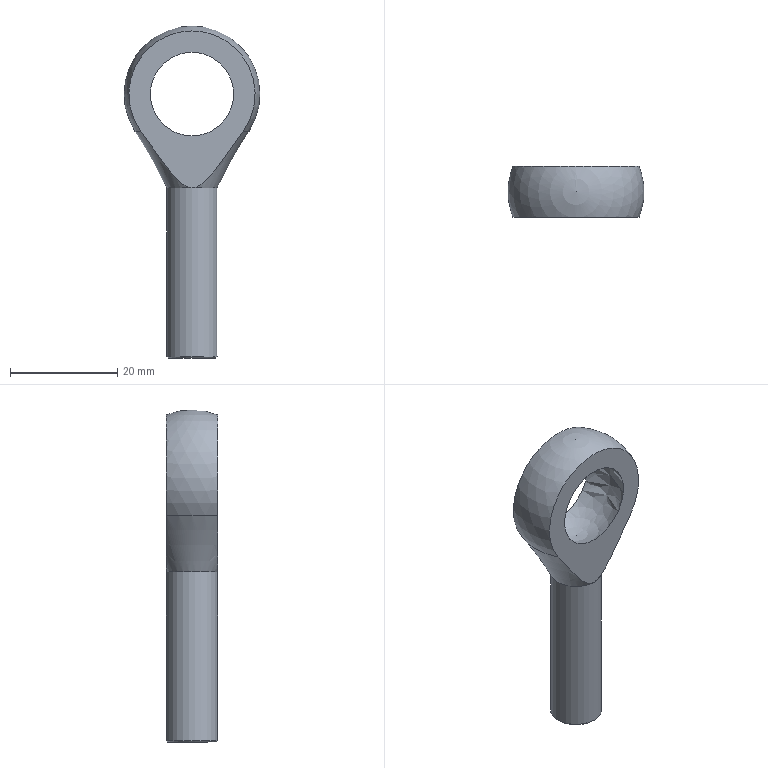Part | NX | features solid 2 | 1 solid | 9 faces | box 25.4 x 9.525 x 61.925 mm | volume 5244 mm3 | plane 3 | torus 2 | sphere 2 | cylinder 1 | cone 1 | commonest cylinder face diameters 9.525 x1
STEP:
#1=CARTESIAN_POINT('',(0.,4.763,-17.475));
#2=VERTEX_POINT('',#1);
#3=CARTESIAN_POINT('',(0.,-4.763,-17.475));
#4=VERTEX_POINT('',#3);
#5=CARTESIAN_POINT('',(0.,0.,-17.475));
#6=DIRECTION('',(0.,0.,-1.));
#7=DIRECTION('',(0.,1.,0.));
#8=AXIS2_PLACEMENT_3D('',#5,#6,#7);
#9=CIRCLE('',#8,4.763);
#10=EDGE_CURVE('',#2,#4,#9,.T.);
#11=ORIENTED_EDGE('',*,*,#10,.F.);
#12=CARTESIAN_POINT('',(9.513,4.763,-6.936));
#13=VERTEX_POINT('',#12);
#14=CARTESIAN_POINT('',(0.,4.763,-17.475));
#15=CARTESIAN_POINT('',(0.618,4.763,-17.475));
#16=CARTESIAN_POINT('',(1.763,4.763,-16.939));
#17=CARTESIAN_POINT('',(3.496,4.763,-15.237));
#18=CARTESIAN_POINT('',(5.308,4.763,-12.838));
#19=CARTESIAN_POINT('',(7.401,4.763,-9.877));
#20=CARTESIAN_POINT('',(8.802,4.763,-7.911));
#21=CARTESIAN_POINT('',(9.513,4.763,-6.936));
#22=B_SPLINE_CURVE_WITH_KNOTS('',3,(#14,#15,#16,#17,#18,#19,#20,#21),.UNSPECIFIED.,.F.,.F.,(4,1,1,1,1,4),(0.,0.001824,0.003648,0.007295,0.01094,0.01459),.UNSPECIFIED.);
#23=EDGE_CURVE('',#2,#13,#22,.T.);
#24=ORIENTED_EDGE('',*,*,#23,.T.);
#25=CARTESIAN_POINT('',(9.513,-4.763,-6.936));
#26=VERTEX_POINT('',#25);
#27=CARTESIAN_POINT('',(0.,0.,-6.936));
#28=DIRECTION('',(0.,0.,-1.));
#29=DIRECTION('',(0.,1.,0.));
#30=AXIS2_PLACEMENT_3D('',#27,#28,#29);
#31=CIRCLE('',#30,10.639);
#32=EDGE_CURVE('',#13,#26,#31,.T.);
#33=ORIENTED_EDGE('',*,*,#32,.T.);
#34=CARTESIAN_POINT('',(9.513,-4.763,-6.936));
#35=CARTESIAN_POINT('',(8.802,-4.763,-7.912));
#36=CARTESIAN_POINT('',(7.398,-4.763,-9.88));
#37=CARTESIAN_POINT('',(5.313,-4.763,-12.837));
#38=CARTESIAN_POINT('',(3.47,-4.763,-15.258));
#39=CARTESIAN_POINT('',(1.776,-4.763,-16.937));
#40=CARTESIAN_POINT('',(0.5927,-4.763,-17.475));
#41=CARTESIAN_POINT('',(0.,-4.763,-17.475));
#42=B_SPLINE_CURVE_WITH_KNOTS('',3,(#34,#35,#36,#37,#38,#39,#40,#41),.UNSPECIFIED.,.F.,.F.,(4,1,1,1,1,4),(0.9357,0.9392,0.9427,0.9462,0.948,0.9497),.UNSPECIFIED.);
#43=EDGE_CURVE('',#26,#4,#42,.T.);
#44=ORIENTED_EDGE('',*,*,#43,.T.);
#45=EDGE_LOOP('',(#11,#24,#33,#44));
#46=FACE_BOUND('',#45,.T.);
#47=CARTESIAN_POINT('',(0.,0.,-54.654));
#48=DIRECTION('',(0.,0.,-1.));
#49=DIRECTION('',(0.,1.,0.));
#50=AXIS2_PLACEMENT_3D('',#47,#48,#49);
#51=DEGENERATE_TOROIDAL_SURFACE('',#50,83.834,87.376,.T.);
#52=ADVANCED_FACE('',(#46),#51,.F.);
#53=CARTESIAN_POINT('',(-9.513,-4.763,-6.936));
#54=VERTEX_POINT('',#53);
#55=CARTESIAN_POINT('',(-9.513,4.763,-6.936));
#56=VERTEX_POINT('',#55);
#57=CARTESIAN_POINT('',(0.,0.,-6.936));
#58=DIRECTION('',(0.,0.,-1.));
#59=DIRECTION('',(0.,1.,0.));
#60=AXIS2_PLACEMENT_3D('',#57,#58,#59);
#61=CIRCLE('',#60,10.639);
#62=EDGE_CURVE('',#54,#56,#61,.T.);
#63=ORIENTED_EDGE('',*,*,#62,.T.);
#64=CARTESIAN_POINT('',(-9.513,4.763,-6.936));
#65=CARTESIAN_POINT('',(-8.802,4.763,-7.912));
#66=CARTESIAN_POINT('',(-7.398,4.763,-9.88));
#67=CARTESIAN_POINT('',(-5.313,4.763,-12.837));
#68=CARTESIAN_POINT('',(-3.47,4.763,-15.258));
#69=CARTESIAN_POINT('',(-1.776,4.763,-16.937));
#70=CARTESIAN_POINT('',(-0.5927,4.763,-17.475));
#71=CARTESIAN_POINT('',(0.,4.763,-17.475));
#72=B_SPLINE_CURVE_WITH_KNOTS('',3,(#64,#65,#66,#67,#68,#69,#70,#71),.UNSPECIFIED.,.F.,.F.,(4,1,1,1,1,4),(0.9357,0.9392,0.9427,0.9462,0.948,0.9497),.UNSPECIFIED.);
#73=EDGE_CURVE('',#56,#2,#72,.T.);
#74=ORIENTED_EDGE('',*,*,#73,.T.);
#75=CARTESIAN_POINT('',(0.,0.,-17.475));
#76=DIRECTION('',(0.,0.,-1.));
#77=DIRECTION('',(0.,1.,0.));
#78=AXIS2_PLACEMENT_3D('',#75,#76,#77);
#79=CIRCLE('',#78,4.763);
#80=EDGE_CURVE('',#4,#2,#79,.T.);
#81=ORIENTED_EDGE('',*,*,#80,.F.);
#82=CARTESIAN_POINT('',(0.,-4.763,-17.475));
#83=CARTESIAN_POINT('',(-0.618,-4.763,-17.475));
#84=CARTESIAN_POINT('',(-1.763,-4.763,-16.939));
#85=CARTESIAN_POINT('',(-3.496,-4.763,-15.237));
#86=CARTESIAN_POINT('',(-5.308,-4.763,-12.838));
#87=CARTESIAN_POINT('',(-7.401,-4.763,-9.877));
#88=CARTESIAN_POINT('',(-8.802,-4.763,-7.911));
#89=CARTESIAN_POINT('',(-9.513,-4.763,-6.936));
#90=B_SPLINE_CURVE_WITH_KNOTS('',3,(#82,#83,#84,#85,#86,#87,#88,#89),.UNSPECIFIED.,.F.,.F.,(4,1,1,1,1,4),(0.,0.001824,0.003648,0.007295,0.01094,0.01459),.UNSPECIFIED.);
#91=EDGE_CURVE('',#4,#54,#90,.T.);
#92=ORIENTED_EDGE('',*,*,#91,.T.);
#93=EDGE_LOOP('',(#63,#74,#81,#92));
#94=FACE_BOUND('',#93,.T.);
#95=CARTESIAN_POINT('',(0.,0.,-54.654));
#96=DIRECTION('',(0.,0.,-1.));
#97=DIRECTION('',(0.,1.,0.));
#98=AXIS2_PLACEMENT_3D('',#95,#96,#97);
#99=DEGENERATE_TOROIDAL_SURFACE('',#98,83.834,87.376,.T.);
#100=ADVANCED_FACE('',(#94),#99,.F.);
#101=ORIENTED_EDGE('',*,*,#32,.F.);
#102=CARTESIAN_POINT('',(0.,4.763,0.));
#103=DIRECTION('',(0.,1.,0.));
#104=DIRECTION('',(0.,0.,1.));
#105=AXIS2_PLACEMENT_3D('',#102,#103,#104);
#106=CIRCLE('',#105,11.773);
#107=EDGE_CURVE('',#13,#56,#106,.F.);
#108=ORIENTED_EDGE('',*,*,#107,.T.);
#109=ORIENTED_EDGE('',*,*,#62,.F.);
#110=CARTESIAN_POINT('',(0.,-4.763,0.));
#111=DIRECTION('',(0.,-1.,0.));
#112=DIRECTION('',(0.,0.,-1.));
#113=AXIS2_PLACEMENT_3D('',#110,#111,#112);
#114=CIRCLE('',#113,11.773);
#115=EDGE_CURVE('',#54,#26,#114,.F.);
#116=ORIENTED_EDGE('',*,*,#115,.T.);
#117=EDGE_LOOP('',(#101,#108,#109,#116));
#118=FACE_BOUND('',#117,.T.);
#119=CARTESIAN_POINT('',(0.,0.,0.));
#120=DIRECTION('',(0.,0.,-1.));
#121=DIRECTION('',(0.,1.,0.));
#122=AXIS2_PLACEMENT_3D('',#119,#120,#121);
#123=SPHERICAL_SURFACE('',#122,12.7);
#124=ADVANCED_FACE('',(#118),#123,.T.);
#125=CARTESIAN_POINT('',(0.,-4.763,-7.776));
#126=VERTEX_POINT('',#125);
#127=CARTESIAN_POINT('',(0.,-4.763,0.));
#128=DIRECTION('',(0.,-1.,0.));
#129=DIRECTION('',(0.,0.,-1.));
#130=AXIS2_PLACEMENT_3D('',#127,#128,#129);
#131=CIRCLE('',#130,7.776);
#132=EDGE_CURVE('',#126,#126,#131,.T.);
#133=ORIENTED_EDGE('',*,*,#132,.T.);
#134=EDGE_LOOP('',(#133));
#135=FACE_BOUND('',#134,.T.);
#136=CARTESIAN_POINT('',(0.,4.763,7.776));
#137=VERTEX_POINT('',#136);
#138=CARTESIAN_POINT('',(0.,4.763,0.));
#139=DIRECTION('',(0.,1.,0.));
#140=DIRECTION('',(0.,0.,1.));
#141=AXIS2_PLACEMENT_3D('',#138,#139,#140);
#142=CIRCLE('',#141,7.776);
#143=EDGE_CURVE('',#137,#137,#142,.T.);
#144=ORIENTED_EDGE('',*,*,#143,.T.);
#145=EDGE_LOOP('',(#144));
#146=FACE_BOUND('',#145,.T.);
#147=CARTESIAN_POINT('',(0.,0.,0.));
#148=DIRECTION('',(0.,0.,-1.));
#149=DIRECTION('',(0.,-1.,0.));
#150=AXIS2_PLACEMENT_3D('',#147,#148,#149);
#151=SPHERICAL_SURFACE('',#150,9.119);
#152=ADVANCED_FACE('',(#135,#146),#151,.F.);
#153=CARTESIAN_POINT('',(0.,4.762,-48.971));
#154=VERTEX_POINT('',#153);
#155=CARTESIAN_POINT('',(0.,0.,-48.971));
#156=DIRECTION('',(0.,0.,-1.));
#157=DIRECTION('',(0.,1.,0.));
#158=AXIS2_PLACEMENT_3D('',#155,#156,#157);
#159=CIRCLE('',#158,4.763);
#160=EDGE_CURVE('',#154,#154,#159,.F.);
#161=ORIENTED_EDGE('',*,*,#160,.T.);
#162=EDGE_LOOP('',(#161));
#163=FACE_BOUND('',#162,.T.);
#164=ORIENTED_EDGE('',*,*,#80,.T.);
#165=ORIENTED_EDGE('',*,*,#10,.T.);
#166=EDGE_LOOP('',(#164,#165));
#167=FACE_BOUND('',#166,.T.);
#168=CARTESIAN_POINT('',(0.,0.,15.494));
#169=DIRECTION('',(0.,0.,-1.));
#170=DIRECTION('',(0.,1.,0.));
#171=AXIS2_PLACEMENT_3D('',#168,#169,#170);
#172=CYLINDRICAL_SURFACE('',#171,4.763);
#173=ADVANCED_FACE('',(#163,#167),#172,.T.);
#174=CARTESIAN_POINT('',(0.,4.508,-49.225));
#175=VERTEX_POINT('',#174);
#176=CARTESIAN_POINT('',(0.,0.,-49.225));
#177=DIRECTION('',(0.,0.,-1.));
#178=DIRECTION('',(0.,1.,0.));
#179=AXIS2_PLACEMENT_3D('',#176,#177,#178);
#180=CIRCLE('',#179,4.508);
#181=EDGE_CURVE('',#175,#175,#180,.T.);
#182=ORIENTED_EDGE('',*,*,#181,.T.);
#183=EDGE_LOOP('',(#182));
#184=FACE_BOUND('',#183,.T.);
#185=CARTESIAN_POINT('',(0.,0.,-49.225));
#186=DIRECTION('',(0.,0.,-1.));
#187=DIRECTION('',(0.,1.,0.));
#188=AXIS2_PLACEMENT_3D('',#185,#186,#187);
#189=PLANE('',#188);
#190=ADVANCED_FACE('',(#184),#189,.T.);
#191=ORIENTED_EDGE('',*,*,#91,.F.);
#192=ORIENTED_EDGE('',*,*,#43,.F.);
#193=ORIENTED_EDGE('',*,*,#115,.F.);
#194=EDGE_LOOP('',(#191,#192,#193));
#195=FACE_BOUND('',#194,.T.);
#196=ORIENTED_EDGE('',*,*,#132,.F.);
#197=EDGE_LOOP('',(#196));
#198=FACE_BOUND('',#197,.T.);
#199=CARTESIAN_POINT('',(0.,-4.763,0.));
#200=DIRECTION('',(0.,-1.,0.));
#201=DIRECTION('',(0.,0.,-1.));
#202=AXIS2_PLACEMENT_3D('',#199,#200,#201);
#203=PLANE('',#202);
#204=ADVANCED_FACE('',(#195,#198),#203,.T.);
#205=ORIENTED_EDGE('',*,*,#23,.F.);
#206=ORIENTED_EDGE('',*,*,#73,.F.);
#207=ORIENTED_EDGE('',*,*,#107,.F.);
#208=EDGE_LOOP('',(#205,#206,#207));
#209=FACE_BOUND('',#208,.T.);
#210=ORIENTED_EDGE('',*,*,#143,.F.);
#211=EDGE_LOOP('',(#210));
#212=FACE_BOUND('',#211,.T.);
#213=CARTESIAN_POINT('',(0.,4.763,0.));
#214=DIRECTION('',(0.,1.,0.));
#215=DIRECTION('',(0.,0.,1.));
#216=AXIS2_PLACEMENT_3D('',#213,#214,#215);
#217=PLANE('',#216);
#218=ADVANCED_FACE('',(#209,#212),#217,.T.);
#219=ORIENTED_EDGE('',*,*,#160,.F.);
#220=EDGE_LOOP('',(#219));
#221=FACE_BOUND('',#220,.T.);
#222=ORIENTED_EDGE('',*,*,#181,.F.);
#223=EDGE_LOOP('',(#222));
#224=FACE_BOUND('',#223,.T.);
#225=CARTESIAN_POINT('',(0.,0.,-49.225));
#226=DIRECTION('',(0.,0.,1.));
#227=DIRECTION('',(0.,-1.,0.));
#228=AXIS2_PLACEMENT_3D('',#225,#226,#227);
#229=CONICAL_SURFACE('',#228,4.508,0.7854);
#230=ADVANCED_FACE('',(#221,#224),#229,.T.);
#231=CLOSED_SHELL('',(#52,#100,#124,#152,#173,#190,#204,#218,#230));
#232=MANIFOLD_SOLID_BREP('',#231);
#233=(LENGTH_UNIT()NAMED_UNIT(*)SI_UNIT(.MILLI.,.METRE.));
#234=UNCERTAINTY_MEASURE_WITH_UNIT(LENGTH_MEASURE(0.0508),#233,'','');
#235=(NAMED_UNIT(*)PLANE_ANGLE_UNIT()SI_UNIT($,.RADIAN.));
#236=(NAMED_UNIT(*)SI_UNIT($,.STERADIAN.)SOLID_ANGLE_UNIT());
#237=(GEOMETRIC_REPRESENTATION_CONTEXT(3)GLOBAL_UNCERTAINTY_ASSIGNED_CONTEXT((#234))GLOBAL_UNIT_ASSIGNED_CONTEXT((#233,#235,#236))REPRESENTATION_CONTEXT('',''));
#238=ADVANCED_BREP_SHAPE_REPRESENTATION('',(#232),#237);